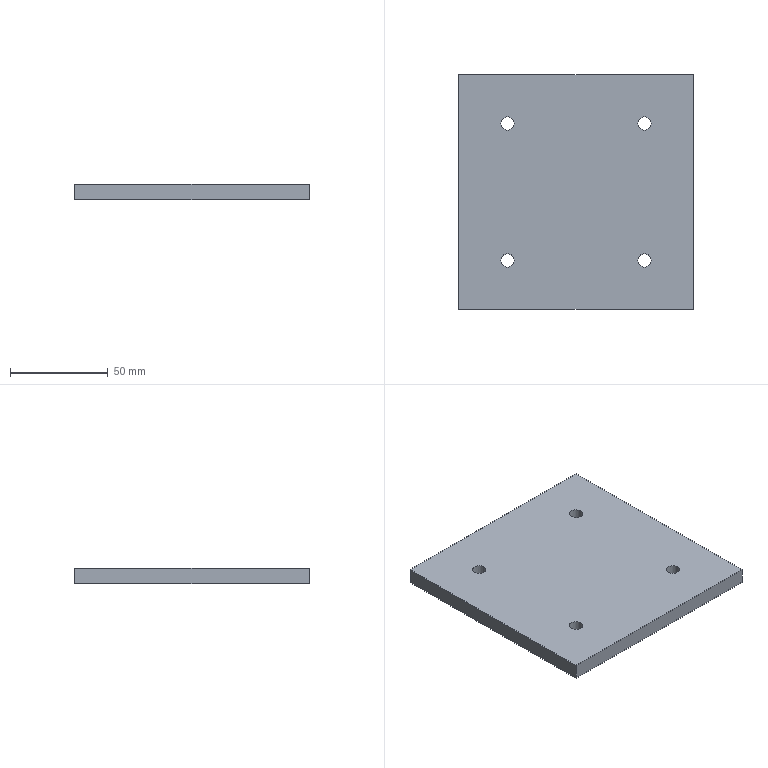Part | STEP file | FHD-021-001-Z Fuma wheel mounting plate | 1 solid | 10 faces | box 120 x 120 x 8 mm | volume 114038 mm3 | plane 6 | cylinder 4 | commonest cylinder face diameters 6.8 x4
STEP:
#1=CARTESIAN_POINT('',(0.,0.,0.));
#2=DIRECTION('',(0.,0.,1.));
#3=DIRECTION('',(1.,0.,0.));
#4=AXIS2_PLACEMENT_3D('',#1,#2,#3);
#5=CARTESIAN_POINT('',(-60.,60.,8.));
#6=VERTEX_POINT('',#5);
#7=CARTESIAN_POINT('',(60.,60.,8.));
#8=VERTEX_POINT('',#7);
#9=CARTESIAN_POINT('',(0.,60.,8.));
#10=DIRECTION('',(1.,0.,0.));
#11=VECTOR('',#10,1.);
#12=LINE('',#9,#11);
#13=CARTESIAN_POINT('',(0.,0.,8.));
#14=DIRECTION('',(0.,0.,-1.));
#15=DIRECTION('',(-1.,0.,0.));
#16=AXIS2_PLACEMENT_3D('',#13,#14,#15);
#17=PLANE('',#16);
#18=CARTESIAN_POINT('',(0.,60.));
#19=DIRECTION('',(-1.,0.));
#20=VECTOR('',#19,1.);
#21=LINE('',#18,#20);
#22=(GEOMETRIC_REPRESENTATION_CONTEXT(2)PARAMETRIC_REPRESENTATION_CONTEXT()REPRESENTATION_CONTEXT('',''));
#23=DEFINITIONAL_REPRESENTATION('',(#21),#22);
#24=PCURVE('',#17,#23);
#25=CARTESIAN_POINT('',(-60.,60.,8.));
#26=DIRECTION('',(0.,-1.,0.));
#27=DIRECTION('',(0.,0.,-1.));
#28=AXIS2_PLACEMENT_3D('',#25,#26,#27);
#29=PLANE('',#28);
#30=CARTESIAN_POINT('',(0.,60.));
#31=DIRECTION('',(0.,1.));
#32=VECTOR('',#31,1.);
#33=LINE('',#30,#32);
#34=(GEOMETRIC_REPRESENTATION_CONTEXT(2)PARAMETRIC_REPRESENTATION_CONTEXT()REPRESENTATION_CONTEXT('',''));
#35=DEFINITIONAL_REPRESENTATION('',(#33),#34);
#36=PCURVE('',#29,#35);
#37=SURFACE_CURVE('',#12,(#24,#36),.PCURVE_S1.);
#38=EDGE_CURVE('',#6,#8,#37,.T.);
#39=ORIENTED_EDGE('',*,*,#38,.F.);
#40=CARTESIAN_POINT('',(-60.,-60.,8.));
#41=VERTEX_POINT('',#40);
#42=CARTESIAN_POINT('',(-60.,0.,8.));
#43=DIRECTION('',(0.,1.,0.));
#44=VECTOR('',#43,1.);
#45=LINE('',#42,#44);
#46=CARTESIAN_POINT('',(60.,0.));
#47=DIRECTION('',(0.,1.));
#48=VECTOR('',#47,1.);
#49=LINE('',#46,#48);
#50=(GEOMETRIC_REPRESENTATION_CONTEXT(2)PARAMETRIC_REPRESENTATION_CONTEXT()REPRESENTATION_CONTEXT('',''));
#51=DEFINITIONAL_REPRESENTATION('',(#49),#50);
#52=PCURVE('',#17,#51);
#53=CARTESIAN_POINT('',(-60.,-60.,8.));
#54=DIRECTION('',(1.,0.,0.));
#55=DIRECTION('',(0.,0.,-1.));
#56=AXIS2_PLACEMENT_3D('',#53,#54,#55);
#57=PLANE('',#56);
#58=CARTESIAN_POINT('',(0.,60.));
#59=DIRECTION('',(0.,1.));
#60=VECTOR('',#59,1.);
#61=LINE('',#58,#60);
#62=(GEOMETRIC_REPRESENTATION_CONTEXT(2)PARAMETRIC_REPRESENTATION_CONTEXT()REPRESENTATION_CONTEXT('',''));
#63=DEFINITIONAL_REPRESENTATION('',(#61),#62);
#64=PCURVE('',#57,#63);
#65=SURFACE_CURVE('',#45,(#52,#64),.PCURVE_S1.);
#66=EDGE_CURVE('',#41,#6,#65,.T.);
#67=ORIENTED_EDGE('',*,*,#66,.F.);
#68=CARTESIAN_POINT('',(60.,-60.,8.));
#69=VERTEX_POINT('',#68);
#70=CARTESIAN_POINT('',(0.,-60.,8.));
#71=DIRECTION('',(-1.,0.,0.));
#72=VECTOR('',#71,1.);
#73=LINE('',#70,#72);
#74=CARTESIAN_POINT('',(0.,-60.));
#75=DIRECTION('',(1.,0.));
#76=VECTOR('',#75,1.);
#77=LINE('',#74,#76);
#78=(GEOMETRIC_REPRESENTATION_CONTEXT(2)PARAMETRIC_REPRESENTATION_CONTEXT()REPRESENTATION_CONTEXT('',''));
#79=DEFINITIONAL_REPRESENTATION('',(#77),#78);
#80=PCURVE('',#17,#79);
#81=CARTESIAN_POINT('',(-60.,-60.,8.));
#82=DIRECTION('',(0.,1.,0.));
#83=DIRECTION('',(0.,0.,1.));
#84=AXIS2_PLACEMENT_3D('',#81,#82,#83);
#85=PLANE('',#84);
#86=CARTESIAN_POINT('',(0.,60.));
#87=DIRECTION('',(0.,-1.));
#88=VECTOR('',#87,1.);
#89=LINE('',#86,#88);
#90=(GEOMETRIC_REPRESENTATION_CONTEXT(2)PARAMETRIC_REPRESENTATION_CONTEXT()REPRESENTATION_CONTEXT('',''));
#91=DEFINITIONAL_REPRESENTATION('',(#89),#90);
#92=PCURVE('',#85,#91);
#93=SURFACE_CURVE('',#73,(#80,#92),.PCURVE_S1.);
#94=EDGE_CURVE('',#69,#41,#93,.T.);
#95=ORIENTED_EDGE('',*,*,#94,.F.);
#96=CARTESIAN_POINT('',(60.,0.,8.));
#97=DIRECTION('',(0.,-1.,0.));
#98=VECTOR('',#97,1.);
#99=LINE('',#96,#98);
#100=CARTESIAN_POINT('',(-60.,0.));
#101=DIRECTION('',(0.,-1.));
#102=VECTOR('',#101,1.);
#103=LINE('',#100,#102);
#104=(GEOMETRIC_REPRESENTATION_CONTEXT(2)PARAMETRIC_REPRESENTATION_CONTEXT()REPRESENTATION_CONTEXT('',''));
#105=DEFINITIONAL_REPRESENTATION('',(#103),#104);
#106=PCURVE('',#17,#105);
#107=CARTESIAN_POINT('',(60.,-60.,8.));
#108=DIRECTION('',(-1.,0.,0.));
#109=DIRECTION('',(0.,0.,1.));
#110=AXIS2_PLACEMENT_3D('',#107,#108,#109);
#111=PLANE('',#110);
#112=CARTESIAN_POINT('',(0.,60.));
#113=DIRECTION('',(0.,-1.));
#114=VECTOR('',#113,1.);
#115=LINE('',#112,#114);
#116=(GEOMETRIC_REPRESENTATION_CONTEXT(2)PARAMETRIC_REPRESENTATION_CONTEXT()REPRESENTATION_CONTEXT('',''));
#117=DEFINITIONAL_REPRESENTATION('',(#115),#116);
#118=PCURVE('',#111,#117);
#119=SURFACE_CURVE('',#99,(#106,#118),.PCURVE_S1.);
#120=EDGE_CURVE('',#8,#69,#119,.T.);
#121=ORIENTED_EDGE('',*,*,#120,.F.);
#122=EDGE_LOOP('',(#39,#67,#95,#121));
#123=FACE_BOUND('',#122,.T.);
#124=CARTESIAN_POINT('',(38.4,-35.,8.));
#125=VERTEX_POINT('',#124);
#126=CARTESIAN_POINT('',(35.,-35.,8.));
#127=DIRECTION('',(0.,0.,1.));
#128=DIRECTION('',(1.,0.,0.));
#129=AXIS2_PLACEMENT_3D('',#126,#127,#128);
#130=CIRCLE('',#129,3.4);
#131=CARTESIAN_POINT('',(-38.4,-35.));
#132=CARTESIAN_POINT('',(-38.4,-29.111));
#133=CARTESIAN_POINT('',(-33.3,-32.056));
#134=CARTESIAN_POINT('',(-28.2,-35.));
#135=CARTESIAN_POINT('',(-33.3,-37.944));
#136=CARTESIAN_POINT('',(-38.4,-40.889));
#137=CARTESIAN_POINT('',(-38.4,-35.));
#138=(BOUNDED_CURVE()B_SPLINE_CURVE(2,(#131,#132,#133,#134,#135,#136,#137),.UNSPECIFIED.,.T.,.F.)B_SPLINE_CURVE_WITH_KNOTS((1,2,2,2,2,1),(-2.094,0.,2.094,4.189,6.283,8.378),.UNSPECIFIED.)CURVE()GEOMETRIC_REPRESENTATION_ITEM()RATIONAL_B_SPLINE_CURVE((1.,0.5,1.,0.5,1.,0.5,1.))REPRESENTATION_ITEM(''));
#139=(GEOMETRIC_REPRESENTATION_CONTEXT(2)PARAMETRIC_REPRESENTATION_CONTEXT()REPRESENTATION_CONTEXT('',''));
#140=DEFINITIONAL_REPRESENTATION('',(#138),#139);
#141=PCURVE('',#17,#140);
#142=CARTESIAN_POINT('',(35.,-35.,8.));
#143=DIRECTION('',(0.,0.,1.));
#144=DIRECTION('',(1.,0.,0.));
#145=AXIS2_PLACEMENT_3D('',#142,#143,#144);
#146=CYLINDRICAL_SURFACE('',#145,3.4);
#147=CARTESIAN_POINT('',(0.,0.));
#148=DIRECTION('',(1.,0.));
#149=VECTOR('',#148,1.);
#150=LINE('',#147,#149);
#151=(GEOMETRIC_REPRESENTATION_CONTEXT(2)PARAMETRIC_REPRESENTATION_CONTEXT()REPRESENTATION_CONTEXT('',''));
#152=DEFINITIONAL_REPRESENTATION('',(#150),#151);
#153=PCURVE('',#146,#152);
#154=SURFACE_CURVE('',#130,(#141,#153),.PCURVE_S1.);
#155=EDGE_CURVE('',#125,#125,#154,.T.);
#156=ORIENTED_EDGE('',*,*,#155,.F.);
#157=EDGE_LOOP('',(#156));
#158=FACE_BOUND('',#157,.T.);
#159=CARTESIAN_POINT('',(38.4,35.,8.));
#160=VERTEX_POINT('',#159);
#161=CARTESIAN_POINT('',(35.,35.,8.));
#162=DIRECTION('',(0.,0.,1.));
#163=DIRECTION('',(1.,0.,0.));
#164=AXIS2_PLACEMENT_3D('',#161,#162,#163);
#165=CIRCLE('',#164,3.4);
#166=CARTESIAN_POINT('',(-38.4,35.));
#167=CARTESIAN_POINT('',(-38.4,40.889));
#168=CARTESIAN_POINT('',(-33.3,37.944));
#169=CARTESIAN_POINT('',(-28.2,35.));
#170=CARTESIAN_POINT('',(-33.3,32.056));
#171=CARTESIAN_POINT('',(-38.4,29.111));
#172=CARTESIAN_POINT('',(-38.4,35.));
#173=(BOUNDED_CURVE()B_SPLINE_CURVE(2,(#166,#167,#168,#169,#170,#171,#172),.UNSPECIFIED.,.T.,.F.)B_SPLINE_CURVE_WITH_KNOTS((1,2,2,2,2,1),(-2.094,0.,2.094,4.189,6.283,8.378),.UNSPECIFIED.)CURVE()GEOMETRIC_REPRESENTATION_ITEM()RATIONAL_B_SPLINE_CURVE((1.,0.5,1.,0.5,1.,0.5,1.))REPRESENTATION_ITEM(''));
#174=(GEOMETRIC_REPRESENTATION_CONTEXT(2)PARAMETRIC_REPRESENTATION_CONTEXT()REPRESENTATION_CONTEXT('',''));
#175=DEFINITIONAL_REPRESENTATION('',(#173),#174);
#176=PCURVE('',#17,#175);
#177=CARTESIAN_POINT('',(35.,35.,8.));
#178=DIRECTION('',(0.,0.,1.));
#179=DIRECTION('',(1.,0.,0.));
#180=AXIS2_PLACEMENT_3D('',#177,#178,#179);
#181=CYLINDRICAL_SURFACE('',#180,3.4);
#182=CARTESIAN_POINT('',(0.,0.));
#183=DIRECTION('',(1.,0.));
#184=VECTOR('',#183,1.);
#185=LINE('',#182,#184);
#186=(GEOMETRIC_REPRESENTATION_CONTEXT(2)PARAMETRIC_REPRESENTATION_CONTEXT()REPRESENTATION_CONTEXT('',''));
#187=DEFINITIONAL_REPRESENTATION('',(#185),#186);
#188=PCURVE('',#181,#187);
#189=SURFACE_CURVE('',#165,(#176,#188),.PCURVE_S1.);
#190=EDGE_CURVE('',#160,#160,#189,.T.);
#191=ORIENTED_EDGE('',*,*,#190,.F.);
#192=EDGE_LOOP('',(#191));
#193=FACE_BOUND('',#192,.T.);
#194=CARTESIAN_POINT('',(-31.6,35.,8.));
#195=VERTEX_POINT('',#194);
#196=CARTESIAN_POINT('',(-35.,35.,8.));
#197=DIRECTION('',(0.,0.,1.));
#198=DIRECTION('',(1.,0.,0.));
#199=AXIS2_PLACEMENT_3D('',#196,#197,#198);
#200=CIRCLE('',#199,3.4);
#201=CARTESIAN_POINT('',(31.6,35.));
#202=CARTESIAN_POINT('',(31.6,40.889));
#203=CARTESIAN_POINT('',(36.7,37.944));
#204=CARTESIAN_POINT('',(41.8,35.));
#205=CARTESIAN_POINT('',(36.7,32.056));
#206=CARTESIAN_POINT('',(31.6,29.111));
#207=CARTESIAN_POINT('',(31.6,35.));
#208=(BOUNDED_CURVE()B_SPLINE_CURVE(2,(#201,#202,#203,#204,#205,#206,#207),.UNSPECIFIED.,.T.,.F.)B_SPLINE_CURVE_WITH_KNOTS((1,2,2,2,2,1),(-2.094,0.,2.094,4.189,6.283,8.378),.UNSPECIFIED.)CURVE()GEOMETRIC_REPRESENTATION_ITEM()RATIONAL_B_SPLINE_CURVE((1.,0.5,1.,0.5,1.,0.5,1.))REPRESENTATION_ITEM(''));
#209=(GEOMETRIC_REPRESENTATION_CONTEXT(2)PARAMETRIC_REPRESENTATION_CONTEXT()REPRESENTATION_CONTEXT('',''));
#210=DEFINITIONAL_REPRESENTATION('',(#208),#209);
#211=PCURVE('',#17,#210);
#212=CARTESIAN_POINT('',(-35.,35.,8.));
#213=DIRECTION('',(0.,0.,1.));
#214=DIRECTION('',(1.,0.,0.));
#215=AXIS2_PLACEMENT_3D('',#212,#213,#214);
#216=CYLINDRICAL_SURFACE('',#215,3.4);
#217=CARTESIAN_POINT('',(0.,0.));
#218=DIRECTION('',(1.,0.));
#219=VECTOR('',#218,1.);
#220=LINE('',#217,#219);
#221=(GEOMETRIC_REPRESENTATION_CONTEXT(2)PARAMETRIC_REPRESENTATION_CONTEXT()REPRESENTATION_CONTEXT('',''));
#222=DEFINITIONAL_REPRESENTATION('',(#220),#221);
#223=PCURVE('',#216,#222);
#224=SURFACE_CURVE('',#200,(#211,#223),.PCURVE_S1.);
#225=EDGE_CURVE('',#195,#195,#224,.T.);
#226=ORIENTED_EDGE('',*,*,#225,.F.);
#227=EDGE_LOOP('',(#226));
#228=FACE_BOUND('',#227,.T.);
#229=CARTESIAN_POINT('',(-31.6,-35.,8.));
#230=VERTEX_POINT('',#229);
#231=CARTESIAN_POINT('',(-35.,-35.,8.));
#232=DIRECTION('',(0.,0.,1.));
#233=DIRECTION('',(1.,0.,0.));
#234=AXIS2_PLACEMENT_3D('',#231,#232,#233);
#235=CIRCLE('',#234,3.4);
#236=CARTESIAN_POINT('',(31.6,-35.));
#237=CARTESIAN_POINT('',(31.6,-29.111));
#238=CARTESIAN_POINT('',(36.7,-32.056));
#239=CARTESIAN_POINT('',(41.8,-35.));
#240=CARTESIAN_POINT('',(36.7,-37.944));
#241=CARTESIAN_POINT('',(31.6,-40.889));
#242=CARTESIAN_POINT('',(31.6,-35.));
#243=(BOUNDED_CURVE()B_SPLINE_CURVE(2,(#236,#237,#238,#239,#240,#241,#242),.UNSPECIFIED.,.T.,.F.)B_SPLINE_CURVE_WITH_KNOTS((1,2,2,2,2,1),(-2.094,0.,2.094,4.189,6.283,8.378),.UNSPECIFIED.)CURVE()GEOMETRIC_REPRESENTATION_ITEM()RATIONAL_B_SPLINE_CURVE((1.,0.5,1.,0.5,1.,0.5,1.))REPRESENTATION_ITEM(''));
#244=(GEOMETRIC_REPRESENTATION_CONTEXT(2)PARAMETRIC_REPRESENTATION_CONTEXT()REPRESENTATION_CONTEXT('',''));
#245=DEFINITIONAL_REPRESENTATION('',(#243),#244);
#246=PCURVE('',#17,#245);
#247=CARTESIAN_POINT('',(-35.,-35.,8.));
#248=DIRECTION('',(0.,0.,1.));
#249=DIRECTION('',(1.,0.,0.));
#250=AXIS2_PLACEMENT_3D('',#247,#248,#249);
#251=CYLINDRICAL_SURFACE('',#250,3.4);
#252=CARTESIAN_POINT('',(0.,0.));
#253=DIRECTION('',(1.,0.));
#254=VECTOR('',#253,1.);
#255=LINE('',#252,#254);
#256=(GEOMETRIC_REPRESENTATION_CONTEXT(2)PARAMETRIC_REPRESENTATION_CONTEXT()REPRESENTATION_CONTEXT('',''));
#257=DEFINITIONAL_REPRESENTATION('',(#255),#256);
#258=PCURVE('',#251,#257);
#259=SURFACE_CURVE('',#235,(#246,#258),.PCURVE_S1.);
#260=EDGE_CURVE('',#230,#230,#259,.T.);
#261=ORIENTED_EDGE('',*,*,#260,.F.);
#262=EDGE_LOOP('',(#261));
#263=FACE_BOUND('',#262,.T.);
#264=ADVANCED_FACE('',(#123,#158,#193,#228,#263),#17,.F.);
#265=CARTESIAN_POINT('',(60.,60.,0.));
#266=VERTEX_POINT('',#265);
#267=CARTESIAN_POINT('',(60.,60.,8.));
#268=DIRECTION('',(0.,0.,-1.));
#269=VECTOR('',#268,1.);
#270=LINE('',#267,#269);
#271=CARTESIAN_POINT('',(0.,120.));
#272=DIRECTION('',(-1.,0.));
#273=VECTOR('',#272,1.);
#274=LINE('',#271,#273);
#275=(GEOMETRIC_REPRESENTATION_CONTEXT(2)PARAMETRIC_REPRESENTATION_CONTEXT()REPRESENTATION_CONTEXT('',''));
#276=DEFINITIONAL_REPRESENTATION('',(#274),#275);
#277=PCURVE('',#111,#276);
#278=CARTESIAN_POINT('',(0.,120.));
#279=DIRECTION('',(1.,0.));
#280=VECTOR('',#279,1.);
#281=LINE('',#278,#280);
#282=(GEOMETRIC_REPRESENTATION_CONTEXT(2)PARAMETRIC_REPRESENTATION_CONTEXT()REPRESENTATION_CONTEXT('',''));
#283=DEFINITIONAL_REPRESENTATION('',(#281),#282);
#284=PCURVE('',#29,#283);
#285=SURFACE_CURVE('',#270,(#277,#284),.PCURVE_S1.);
#286=EDGE_CURVE('',#8,#266,#285,.T.);
#287=ORIENTED_EDGE('',*,*,#286,.F.);
#288=ORIENTED_EDGE('',*,*,#120,.T.);
#289=CARTESIAN_POINT('',(60.,-60.,0.));
#290=VERTEX_POINT('',#289);
#291=CARTESIAN_POINT('',(60.,-60.,8.));
#292=DIRECTION('',(0.,0.,1.));
#293=VECTOR('',#292,1.);
#294=LINE('',#291,#293);
#295=CARTESIAN_POINT('',(0.,0.));
#296=DIRECTION('',(1.,0.));
#297=VECTOR('',#296,1.);
#298=LINE('',#295,#297);
#299=(GEOMETRIC_REPRESENTATION_CONTEXT(2)PARAMETRIC_REPRESENTATION_CONTEXT()REPRESENTATION_CONTEXT('',''));
#300=DEFINITIONAL_REPRESENTATION('',(#298),#299);
#301=PCURVE('',#111,#300);
#302=CARTESIAN_POINT('',(0.,120.));
#303=DIRECTION('',(1.,0.));
#304=VECTOR('',#303,1.);
#305=LINE('',#302,#304);
#306=(GEOMETRIC_REPRESENTATION_CONTEXT(2)PARAMETRIC_REPRESENTATION_CONTEXT()REPRESENTATION_CONTEXT('',''));
#307=DEFINITIONAL_REPRESENTATION('',(#305),#306);
#308=PCURVE('',#85,#307);
#309=SURFACE_CURVE('',#294,(#301,#308),.PCURVE_S1.);
#310=EDGE_CURVE('',#290,#69,#309,.T.);
#311=ORIENTED_EDGE('',*,*,#310,.F.);
#312=CARTESIAN_POINT('',(60.,-60.,0.));
#313=DIRECTION('',(0.,-1.,0.));
#314=VECTOR('',#313,1.);
#315=LINE('',#312,#314);
#316=CARTESIAN_POINT('',(-8.,0.));
#317=DIRECTION('',(0.,-1.));
#318=VECTOR('',#317,1.);
#319=LINE('',#316,#318);
#320=(GEOMETRIC_REPRESENTATION_CONTEXT(2)PARAMETRIC_REPRESENTATION_CONTEXT()REPRESENTATION_CONTEXT('',''));
#321=DEFINITIONAL_REPRESENTATION('',(#319),#320);
#322=PCURVE('',#111,#321);
#323=CARTESIAN_POINT('',(0.,0.,0.));
#324=DIRECTION('',(0.,0.,-1.));
#325=DIRECTION('',(-1.,0.,0.));
#326=AXIS2_PLACEMENT_3D('',#323,#324,#325);
#327=PLANE('',#326);
#328=CARTESIAN_POINT('',(-60.,-60.));
#329=DIRECTION('',(0.,-1.));
#330=VECTOR('',#329,1.);
#331=LINE('',#328,#330);
#332=(GEOMETRIC_REPRESENTATION_CONTEXT(2)PARAMETRIC_REPRESENTATION_CONTEXT()REPRESENTATION_CONTEXT('',''));
#333=DEFINITIONAL_REPRESENTATION('',(#331),#332);
#334=PCURVE('',#327,#333);
#335=SURFACE_CURVE('',#315,(#322,#334),.PCURVE_S1.);
#336=EDGE_CURVE('',#266,#290,#335,.T.);
#337=ORIENTED_EDGE('',*,*,#336,.F.);
#338=EDGE_LOOP('',(#287,#288,#311,#337));
#339=FACE_BOUND('',#338,.T.);
#340=ADVANCED_FACE('',(#339),#111,.F.);
#341=CARTESIAN_POINT('',(-60.,60.,0.));
#342=VERTEX_POINT('',#341);
#343=CARTESIAN_POINT('',(-60.,60.,8.));
#344=DIRECTION('',(0.,0.,-1.));
#345=VECTOR('',#344,1.);
#346=LINE('',#343,#345);
#347=CARTESIAN_POINT('',(0.,0.));
#348=DIRECTION('',(1.,0.));
#349=VECTOR('',#348,1.);
#350=LINE('',#347,#349);
#351=(GEOMETRIC_REPRESENTATION_CONTEXT(2)PARAMETRIC_REPRESENTATION_CONTEXT()REPRESENTATION_CONTEXT('',''));
#352=DEFINITIONAL_REPRESENTATION('',(#350),#351);
#353=PCURVE('',#29,#352);
#354=CARTESIAN_POINT('',(0.,120.));
#355=DIRECTION('',(1.,0.));
#356=VECTOR('',#355,1.);
#357=LINE('',#354,#356);
#358=(GEOMETRIC_REPRESENTATION_CONTEXT(2)PARAMETRIC_REPRESENTATION_CONTEXT()REPRESENTATION_CONTEXT('',''));
#359=DEFINITIONAL_REPRESENTATION('',(#357),#358);
#360=PCURVE('',#57,#359);
#361=SURFACE_CURVE('',#346,(#353,#360),.PCURVE_S1.);
#362=EDGE_CURVE('',#6,#342,#361,.T.);
#363=ORIENTED_EDGE('',*,*,#362,.F.);
#364=ORIENTED_EDGE('',*,*,#38,.T.);
#365=ORIENTED_EDGE('',*,*,#286,.T.);
#366=CARTESIAN_POINT('',(-60.,60.,0.));
#367=DIRECTION('',(1.,0.,0.));
#368=VECTOR('',#367,1.);
#369=LINE('',#366,#368);
#370=CARTESIAN_POINT('',(8.,0.));
#371=DIRECTION('',(0.,1.));
#372=VECTOR('',#371,1.);
#373=LINE('',#370,#372);
#374=(GEOMETRIC_REPRESENTATION_CONTEXT(2)PARAMETRIC_REPRESENTATION_CONTEXT()REPRESENTATION_CONTEXT('',''));
#375=DEFINITIONAL_REPRESENTATION('',(#373),#374);
#376=PCURVE('',#29,#375);
#377=CARTESIAN_POINT('',(60.,60.));
#378=DIRECTION('',(-1.,0.));
#379=VECTOR('',#378,1.);
#380=LINE('',#377,#379);
#381=(GEOMETRIC_REPRESENTATION_CONTEXT(2)PARAMETRIC_REPRESENTATION_CONTEXT()REPRESENTATION_CONTEXT('',''));
#382=DEFINITIONAL_REPRESENTATION('',(#380),#381);
#383=PCURVE('',#327,#382);
#384=SURFACE_CURVE('',#369,(#376,#383),.PCURVE_S1.);
#385=EDGE_CURVE('',#342,#266,#384,.T.);
#386=ORIENTED_EDGE('',*,*,#385,.F.);
#387=EDGE_LOOP('',(#363,#364,#365,#386));
#388=FACE_BOUND('',#387,.T.);
#389=ADVANCED_FACE('',(#388),#29,.F.);
#390=CARTESIAN_POINT('',(-60.,-60.,0.));
#391=VERTEX_POINT('',#390);
#392=CARTESIAN_POINT('',(-60.,-60.,8.));
#393=DIRECTION('',(0.,0.,-1.));
#394=VECTOR('',#393,1.);
#395=LINE('',#392,#394);
#396=CARTESIAN_POINT('',(0.,0.));
#397=DIRECTION('',(1.,0.));
#398=VECTOR('',#397,1.);
#399=LINE('',#396,#398);
#400=(GEOMETRIC_REPRESENTATION_CONTEXT(2)PARAMETRIC_REPRESENTATION_CONTEXT()REPRESENTATION_CONTEXT('',''));
#401=DEFINITIONAL_REPRESENTATION('',(#399),#400);
#402=PCURVE('',#57,#401);
#403=CARTESIAN_POINT('',(0.,0.));
#404=DIRECTION('',(-1.,0.));
#405=VECTOR('',#404,1.);
#406=LINE('',#403,#405);
#407=(GEOMETRIC_REPRESENTATION_CONTEXT(2)PARAMETRIC_REPRESENTATION_CONTEXT()REPRESENTATION_CONTEXT('',''));
#408=DEFINITIONAL_REPRESENTATION('',(#406),#407);
#409=PCURVE('',#85,#408);
#410=SURFACE_CURVE('',#395,(#402,#409),.PCURVE_S1.);
#411=EDGE_CURVE('',#41,#391,#410,.T.);
#412=ORIENTED_EDGE('',*,*,#411,.F.);
#413=ORIENTED_EDGE('',*,*,#66,.T.);
#414=ORIENTED_EDGE('',*,*,#362,.T.);
#415=CARTESIAN_POINT('',(-60.,-60.,0.));
#416=DIRECTION('',(0.,1.,0.));
#417=VECTOR('',#416,1.);
#418=LINE('',#415,#417);
#419=CARTESIAN_POINT('',(8.,0.));
#420=DIRECTION('',(0.,1.));
#421=VECTOR('',#420,1.);
#422=LINE('',#419,#421);
#423=(GEOMETRIC_REPRESENTATION_CONTEXT(2)PARAMETRIC_REPRESENTATION_CONTEXT()REPRESENTATION_CONTEXT('',''));
#424=DEFINITIONAL_REPRESENTATION('',(#422),#423);
#425=PCURVE('',#57,#424);
#426=CARTESIAN_POINT('',(60.,-60.));
#427=DIRECTION('',(0.,1.));
#428=VECTOR('',#427,1.);
#429=LINE('',#426,#428);
#430=(GEOMETRIC_REPRESENTATION_CONTEXT(2)PARAMETRIC_REPRESENTATION_CONTEXT()REPRESENTATION_CONTEXT('',''));
#431=DEFINITIONAL_REPRESENTATION('',(#429),#430);
#432=PCURVE('',#327,#431);
#433=SURFACE_CURVE('',#418,(#425,#432),.PCURVE_S1.);
#434=EDGE_CURVE('',#391,#342,#433,.T.);
#435=ORIENTED_EDGE('',*,*,#434,.F.);
#436=EDGE_LOOP('',(#412,#413,#414,#435));
#437=FACE_BOUND('',#436,.T.);
#438=ADVANCED_FACE('',(#437),#57,.F.);
#439=ORIENTED_EDGE('',*,*,#310,.T.);
#440=ORIENTED_EDGE('',*,*,#94,.T.);
#441=ORIENTED_EDGE('',*,*,#411,.T.);
#442=CARTESIAN_POINT('',(-60.,-60.,0.));
#443=DIRECTION('',(-1.,0.,0.));
#444=VECTOR('',#443,1.);
#445=LINE('',#442,#444);
#446=CARTESIAN_POINT('',(-8.,0.));
#447=DIRECTION('',(0.,-1.));
#448=VECTOR('',#447,1.);
#449=LINE('',#446,#448);
#450=(GEOMETRIC_REPRESENTATION_CONTEXT(2)PARAMETRIC_REPRESENTATION_CONTEXT()REPRESENTATION_CONTEXT('',''));
#451=DEFINITIONAL_REPRESENTATION('',(#449),#450);
#452=PCURVE('',#85,#451);
#453=CARTESIAN_POINT('',(60.,-60.));
#454=DIRECTION('',(1.,0.));
#455=VECTOR('',#454,1.);
#456=LINE('',#453,#455);
#457=(GEOMETRIC_REPRESENTATION_CONTEXT(2)PARAMETRIC_REPRESENTATION_CONTEXT()REPRESENTATION_CONTEXT('',''));
#458=DEFINITIONAL_REPRESENTATION('',(#456),#457);
#459=PCURVE('',#327,#458);
#460=SURFACE_CURVE('',#445,(#452,#459),.PCURVE_S1.);
#461=EDGE_CURVE('',#290,#391,#460,.T.);
#462=ORIENTED_EDGE('',*,*,#461,.F.);
#463=EDGE_LOOP('',(#439,#440,#441,#462));
#464=FACE_BOUND('',#463,.T.);
#465=ADVANCED_FACE('',(#464),#85,.F.);
#466=CARTESIAN_POINT('',(38.4,-35.,0.));
#467=VERTEX_POINT('',#466);
#468=CARTESIAN_POINT('',(35.,-35.,0.));
#469=DIRECTION('',(0.,0.,1.));
#470=DIRECTION('',(1.,0.,0.));
#471=AXIS2_PLACEMENT_3D('',#468,#469,#470);
#472=CIRCLE('',#471,3.4);
#473=CARTESIAN_POINT('',(0.,-8.));
#474=DIRECTION('',(1.,0.));
#475=VECTOR('',#474,1.);
#476=LINE('',#473,#475);
#477=(GEOMETRIC_REPRESENTATION_CONTEXT(2)PARAMETRIC_REPRESENTATION_CONTEXT()REPRESENTATION_CONTEXT('',''));
#478=DEFINITIONAL_REPRESENTATION('',(#476),#477);
#479=PCURVE('',#146,#478);
#480=CARTESIAN_POINT('',(-38.4,-35.));
#481=CARTESIAN_POINT('',(-38.4,-29.111));
#482=CARTESIAN_POINT('',(-33.3,-32.056));
#483=CARTESIAN_POINT('',(-28.2,-35.));
#484=CARTESIAN_POINT('',(-33.3,-37.944));
#485=CARTESIAN_POINT('',(-38.4,-40.889));
#486=CARTESIAN_POINT('',(-38.4,-35.));
#487=(BOUNDED_CURVE()B_SPLINE_CURVE(2,(#480,#481,#482,#483,#484,#485,#486),.UNSPECIFIED.,.T.,.F.)B_SPLINE_CURVE_WITH_KNOTS((1,2,2,2,2,1),(-2.094,0.,2.094,4.189,6.283,8.378),.UNSPECIFIED.)CURVE()GEOMETRIC_REPRESENTATION_ITEM()RATIONAL_B_SPLINE_CURVE((1.,0.5,1.,0.5,1.,0.5,1.))REPRESENTATION_ITEM(''));
#488=(GEOMETRIC_REPRESENTATION_CONTEXT(2)PARAMETRIC_REPRESENTATION_CONTEXT()REPRESENTATION_CONTEXT('',''));
#489=DEFINITIONAL_REPRESENTATION('',(#487),#488);
#490=PCURVE('',#327,#489);
#491=SURFACE_CURVE('',#472,(#479,#490),.PCURVE_S1.);
#492=EDGE_CURVE('',#467,#467,#491,.T.);
#493=ORIENTED_EDGE('',*,*,#492,.T.);
#494=CARTESIAN_POINT('',(38.4,-35.,0.));
#495=CARTESIAN_POINT('',(38.4,-35.,8.));
#496=B_SPLINE_CURVE_WITH_KNOTS('',1,(#494,#495),.UNSPECIFIED.,.F.,.F.,(2,2),(-8.,0.),.PIECEWISE_BEZIER_KNOTS.);
#497=CARTESIAN_POINT('',(6.283,0.));
#498=DIRECTION('',(0.,1.));
#499=VECTOR('',#498,1.);
#500=LINE('',#497,#499);
#501=(GEOMETRIC_REPRESENTATION_CONTEXT(2)PARAMETRIC_REPRESENTATION_CONTEXT()REPRESENTATION_CONTEXT('',''));
#502=DEFINITIONAL_REPRESENTATION('',(#500),#501);
#503=PCURVE('',#146,#502);
#504=CARTESIAN_POINT('',(0.,0.));
#505=DIRECTION('',(0.,1.));
#506=VECTOR('',#505,1.);
#507=LINE('',#504,#506);
#508=(GEOMETRIC_REPRESENTATION_CONTEXT(2)PARAMETRIC_REPRESENTATION_CONTEXT()REPRESENTATION_CONTEXT('',''));
#509=DEFINITIONAL_REPRESENTATION('',(#507),#508);
#510=PCURVE('',#146,#509);
#511=SEAM_CURVE('',#496,(#503,#510),.PCURVE_S1.);
#512=EDGE_CURVE('',#467,#125,#511,.T.);
#513=ORIENTED_EDGE('',*,*,#512,.T.);
#514=ORIENTED_EDGE('',*,*,#155,.F.);
#515=ORIENTED_EDGE('',*,*,#512,.F.);
#516=EDGE_LOOP('',(#493,#513,#514,#515));
#517=FACE_BOUND('',#516,.F.);
#518=ADVANCED_FACE('',(#517),#146,.F.);
#519=CARTESIAN_POINT('',(38.4,35.,0.));
#520=VERTEX_POINT('',#519);
#521=CARTESIAN_POINT('',(35.,35.,0.));
#522=DIRECTION('',(0.,0.,1.));
#523=DIRECTION('',(1.,0.,0.));
#524=AXIS2_PLACEMENT_3D('',#521,#522,#523);
#525=CIRCLE('',#524,3.4);
#526=CARTESIAN_POINT('',(0.,-8.));
#527=DIRECTION('',(1.,0.));
#528=VECTOR('',#527,1.);
#529=LINE('',#526,#528);
#530=(GEOMETRIC_REPRESENTATION_CONTEXT(2)PARAMETRIC_REPRESENTATION_CONTEXT()REPRESENTATION_CONTEXT('',''));
#531=DEFINITIONAL_REPRESENTATION('',(#529),#530);
#532=PCURVE('',#181,#531);
#533=CARTESIAN_POINT('',(-38.4,35.));
#534=CARTESIAN_POINT('',(-38.4,40.889));
#535=CARTESIAN_POINT('',(-33.3,37.944));
#536=CARTESIAN_POINT('',(-28.2,35.));
#537=CARTESIAN_POINT('',(-33.3,32.056));
#538=CARTESIAN_POINT('',(-38.4,29.111));
#539=CARTESIAN_POINT('',(-38.4,35.));
#540=(BOUNDED_CURVE()B_SPLINE_CURVE(2,(#533,#534,#535,#536,#537,#538,#539),.UNSPECIFIED.,.T.,.F.)B_SPLINE_CURVE_WITH_KNOTS((1,2,2,2,2,1),(-2.094,0.,2.094,4.189,6.283,8.378),.UNSPECIFIED.)CURVE()GEOMETRIC_REPRESENTATION_ITEM()RATIONAL_B_SPLINE_CURVE((1.,0.5,1.,0.5,1.,0.5,1.))REPRESENTATION_ITEM(''));
#541=(GEOMETRIC_REPRESENTATION_CONTEXT(2)PARAMETRIC_REPRESENTATION_CONTEXT()REPRESENTATION_CONTEXT('',''));
#542=DEFINITIONAL_REPRESENTATION('',(#540),#541);
#543=PCURVE('',#327,#542);
#544=SURFACE_CURVE('',#525,(#532,#543),.PCURVE_S1.);
#545=EDGE_CURVE('',#520,#520,#544,.T.);
#546=ORIENTED_EDGE('',*,*,#545,.T.);
#547=CARTESIAN_POINT('',(38.4,35.,0.));
#548=CARTESIAN_POINT('',(38.4,35.,8.));
#549=B_SPLINE_CURVE_WITH_KNOTS('',1,(#547,#548),.UNSPECIFIED.,.F.,.F.,(2,2),(-8.,0.),.PIECEWISE_BEZIER_KNOTS.);
#550=CARTESIAN_POINT('',(6.283,0.));
#551=DIRECTION('',(0.,1.));
#552=VECTOR('',#551,1.);
#553=LINE('',#550,#552);
#554=(GEOMETRIC_REPRESENTATION_CONTEXT(2)PARAMETRIC_REPRESENTATION_CONTEXT()REPRESENTATION_CONTEXT('',''));
#555=DEFINITIONAL_REPRESENTATION('',(#553),#554);
#556=PCURVE('',#181,#555);
#557=CARTESIAN_POINT('',(0.,0.));
#558=DIRECTION('',(0.,1.));
#559=VECTOR('',#558,1.);
#560=LINE('',#557,#559);
#561=(GEOMETRIC_REPRESENTATION_CONTEXT(2)PARAMETRIC_REPRESENTATION_CONTEXT()REPRESENTATION_CONTEXT('',''));
#562=DEFINITIONAL_REPRESENTATION('',(#560),#561);
#563=PCURVE('',#181,#562);
#564=SEAM_CURVE('',#549,(#556,#563),.PCURVE_S1.);
#565=EDGE_CURVE('',#520,#160,#564,.T.);
#566=ORIENTED_EDGE('',*,*,#565,.T.);
#567=ORIENTED_EDGE('',*,*,#190,.F.);
#568=ORIENTED_EDGE('',*,*,#565,.F.);
#569=EDGE_LOOP('',(#546,#566,#567,#568));
#570=FACE_BOUND('',#569,.F.);
#571=ADVANCED_FACE('',(#570),#181,.F.);
#572=CARTESIAN_POINT('',(-31.6,35.,0.));
#573=VERTEX_POINT('',#572);
#574=CARTESIAN_POINT('',(-35.,35.,0.));
#575=DIRECTION('',(0.,0.,1.));
#576=DIRECTION('',(1.,0.,0.));
#577=AXIS2_PLACEMENT_3D('',#574,#575,#576);
#578=CIRCLE('',#577,3.4);
#579=CARTESIAN_POINT('',(0.,-8.));
#580=DIRECTION('',(1.,0.));
#581=VECTOR('',#580,1.);
#582=LINE('',#579,#581);
#583=(GEOMETRIC_REPRESENTATION_CONTEXT(2)PARAMETRIC_REPRESENTATION_CONTEXT()REPRESENTATION_CONTEXT('',''));
#584=DEFINITIONAL_REPRESENTATION('',(#582),#583);
#585=PCURVE('',#216,#584);
#586=CARTESIAN_POINT('',(31.6,35.));
#587=CARTESIAN_POINT('',(31.6,40.889));
#588=CARTESIAN_POINT('',(36.7,37.944));
#589=CARTESIAN_POINT('',(41.8,35.));
#590=CARTESIAN_POINT('',(36.7,32.056));
#591=CARTESIAN_POINT('',(31.6,29.111));
#592=CARTESIAN_POINT('',(31.6,35.));
#593=(BOUNDED_CURVE()B_SPLINE_CURVE(2,(#586,#587,#588,#589,#590,#591,#592),.UNSPECIFIED.,.T.,.F.)B_SPLINE_CURVE_WITH_KNOTS((1,2,2,2,2,1),(-2.094,0.,2.094,4.189,6.283,8.378),.UNSPECIFIED.)CURVE()GEOMETRIC_REPRESENTATION_ITEM()RATIONAL_B_SPLINE_CURVE((1.,0.5,1.,0.5,1.,0.5,1.))REPRESENTATION_ITEM(''));
#594=(GEOMETRIC_REPRESENTATION_CONTEXT(2)PARAMETRIC_REPRESENTATION_CONTEXT()REPRESENTATION_CONTEXT('',''));
#595=DEFINITIONAL_REPRESENTATION('',(#593),#594);
#596=PCURVE('',#327,#595);
#597=SURFACE_CURVE('',#578,(#585,#596),.PCURVE_S1.);
#598=EDGE_CURVE('',#573,#573,#597,.T.);
#599=ORIENTED_EDGE('',*,*,#598,.T.);
#600=CARTESIAN_POINT('',(-31.6,35.,0.));
#601=CARTESIAN_POINT('',(-31.6,35.,8.));
#602=B_SPLINE_CURVE_WITH_KNOTS('',1,(#600,#601),.UNSPECIFIED.,.F.,.F.,(2,2),(-8.,0.),.PIECEWISE_BEZIER_KNOTS.);
#603=CARTESIAN_POINT('',(6.283,0.));
#604=DIRECTION('',(0.,1.));
#605=VECTOR('',#604,1.);
#606=LINE('',#603,#605);
#607=(GEOMETRIC_REPRESENTATION_CONTEXT(2)PARAMETRIC_REPRESENTATION_CONTEXT()REPRESENTATION_CONTEXT('',''));
#608=DEFINITIONAL_REPRESENTATION('',(#606),#607);
#609=PCURVE('',#216,#608);
#610=CARTESIAN_POINT('',(0.,0.));
#611=DIRECTION('',(0.,1.));
#612=VECTOR('',#611,1.);
#613=LINE('',#610,#612);
#614=(GEOMETRIC_REPRESENTATION_CONTEXT(2)PARAMETRIC_REPRESENTATION_CONTEXT()REPRESENTATION_CONTEXT('',''));
#615=DEFINITIONAL_REPRESENTATION('',(#613),#614);
#616=PCURVE('',#216,#615);
#617=SEAM_CURVE('',#602,(#609,#616),.PCURVE_S1.);
#618=EDGE_CURVE('',#573,#195,#617,.T.);
#619=ORIENTED_EDGE('',*,*,#618,.T.);
#620=ORIENTED_EDGE('',*,*,#225,.F.);
#621=ORIENTED_EDGE('',*,*,#618,.F.);
#622=EDGE_LOOP('',(#599,#619,#620,#621));
#623=FACE_BOUND('',#622,.F.);
#624=ADVANCED_FACE('',(#623),#216,.F.);
#625=CARTESIAN_POINT('',(-31.6,-35.,0.));
#626=VERTEX_POINT('',#625);
#627=CARTESIAN_POINT('',(-35.,-35.,0.));
#628=DIRECTION('',(0.,0.,1.));
#629=DIRECTION('',(1.,0.,0.));
#630=AXIS2_PLACEMENT_3D('',#627,#628,#629);
#631=CIRCLE('',#630,3.4);
#632=CARTESIAN_POINT('',(0.,-8.));
#633=DIRECTION('',(1.,0.));
#634=VECTOR('',#633,1.);
#635=LINE('',#632,#634);
#636=(GEOMETRIC_REPRESENTATION_CONTEXT(2)PARAMETRIC_REPRESENTATION_CONTEXT()REPRESENTATION_CONTEXT('',''));
#637=DEFINITIONAL_REPRESENTATION('',(#635),#636);
#638=PCURVE('',#251,#637);
#639=CARTESIAN_POINT('',(31.6,-35.));
#640=CARTESIAN_POINT('',(31.6,-29.111));
#641=CARTESIAN_POINT('',(36.7,-32.056));
#642=CARTESIAN_POINT('',(41.8,-35.));
#643=CARTESIAN_POINT('',(36.7,-37.944));
#644=CARTESIAN_POINT('',(31.6,-40.889));
#645=CARTESIAN_POINT('',(31.6,-35.));
#646=(BOUNDED_CURVE()B_SPLINE_CURVE(2,(#639,#640,#641,#642,#643,#644,#645),.UNSPECIFIED.,.T.,.F.)B_SPLINE_CURVE_WITH_KNOTS((1,2,2,2,2,1),(-2.094,0.,2.094,4.189,6.283,8.378),.UNSPECIFIED.)CURVE()GEOMETRIC_REPRESENTATION_ITEM()RATIONAL_B_SPLINE_CURVE((1.,0.5,1.,0.5,1.,0.5,1.))REPRESENTATION_ITEM(''));
#647=(GEOMETRIC_REPRESENTATION_CONTEXT(2)PARAMETRIC_REPRESENTATION_CONTEXT()REPRESENTATION_CONTEXT('',''));
#648=DEFINITIONAL_REPRESENTATION('',(#646),#647);
#649=PCURVE('',#327,#648);
#650=SURFACE_CURVE('',#631,(#638,#649),.PCURVE_S1.);
#651=EDGE_CURVE('',#626,#626,#650,.T.);
#652=ORIENTED_EDGE('',*,*,#651,.T.);
#653=CARTESIAN_POINT('',(-31.6,-35.,0.));
#654=CARTESIAN_POINT('',(-31.6,-35.,8.));
#655=B_SPLINE_CURVE_WITH_KNOTS('',1,(#653,#654),.UNSPECIFIED.,.F.,.F.,(2,2),(-8.,0.),.PIECEWISE_BEZIER_KNOTS.);
#656=CARTESIAN_POINT('',(6.283,0.));
#657=DIRECTION('',(0.,1.));
#658=VECTOR('',#657,1.);
#659=LINE('',#656,#658);
#660=(GEOMETRIC_REPRESENTATION_CONTEXT(2)PARAMETRIC_REPRESENTATION_CONTEXT()REPRESENTATION_CONTEXT('',''));
#661=DEFINITIONAL_REPRESENTATION('',(#659),#660);
#662=PCURVE('',#251,#661);
#663=CARTESIAN_POINT('',(0.,0.));
#664=DIRECTION('',(0.,1.));
#665=VECTOR('',#664,1.);
#666=LINE('',#663,#665);
#667=(GEOMETRIC_REPRESENTATION_CONTEXT(2)PARAMETRIC_REPRESENTATION_CONTEXT()REPRESENTATION_CONTEXT('',''));
#668=DEFINITIONAL_REPRESENTATION('',(#666),#667);
#669=PCURVE('',#251,#668);
#670=SEAM_CURVE('',#655,(#662,#669),.PCURVE_S1.);
#671=EDGE_CURVE('',#626,#230,#670,.T.);
#672=ORIENTED_EDGE('',*,*,#671,.T.);
#673=ORIENTED_EDGE('',*,*,#260,.F.);
#674=ORIENTED_EDGE('',*,*,#671,.F.);
#675=EDGE_LOOP('',(#652,#672,#673,#674));
#676=FACE_BOUND('',#675,.F.);
#677=ADVANCED_FACE('',(#676),#251,.F.);
#678=ORIENTED_EDGE('',*,*,#434,.T.);
#679=ORIENTED_EDGE('',*,*,#385,.T.);
#680=ORIENTED_EDGE('',*,*,#336,.T.);
#681=ORIENTED_EDGE('',*,*,#461,.T.);
#682=EDGE_LOOP('',(#678,#679,#680,#681));
#683=FACE_BOUND('',#682,.T.);
#684=ORIENTED_EDGE('',*,*,#492,.T.);
#685=EDGE_LOOP('',(#684));
#686=FACE_BOUND('',#685,.T.);
#687=ORIENTED_EDGE('',*,*,#545,.T.);
#688=EDGE_LOOP('',(#687));
#689=FACE_BOUND('',#688,.T.);
#690=ORIENTED_EDGE('',*,*,#598,.T.);
#691=EDGE_LOOP('',(#690));
#692=FACE_BOUND('',#691,.T.);
#693=ORIENTED_EDGE('',*,*,#651,.T.);
#694=EDGE_LOOP('',(#693));
#695=FACE_BOUND('',#694,.T.);
#696=ADVANCED_FACE('',(#683,#686,#689,#692,#695),#327,.T.);
#697=CLOSED_SHELL('',(#264,#340,#389,#438,#465,#518,#571,#624,#677,#696));
#698=MANIFOLD_SOLID_BREP('',#697);
#699=(LENGTH_UNIT()NAMED_UNIT(*)SI_UNIT(.MILLI.,.METRE.));
#700=UNCERTAINTY_MEASURE_WITH_UNIT(LENGTH_MEASURE(0.000005),#699,'','');
#701=(NAMED_UNIT(*)PLANE_ANGLE_UNIT()SI_UNIT($,.RADIAN.));
#702=(NAMED_UNIT(*)SI_UNIT($,.STERADIAN.)SOLID_ANGLE_UNIT());
#703=(GEOMETRIC_REPRESENTATION_CONTEXT(3)GLOBAL_UNCERTAINTY_ASSIGNED_CONTEXT((#700))GLOBAL_UNIT_ASSIGNED_CONTEXT((#699,#701,#702))REPRESENTATION_CONTEXT('',''));
#704=ADVANCED_BREP_SHAPE_REPRESENTATION('',(#4,#698),#703);